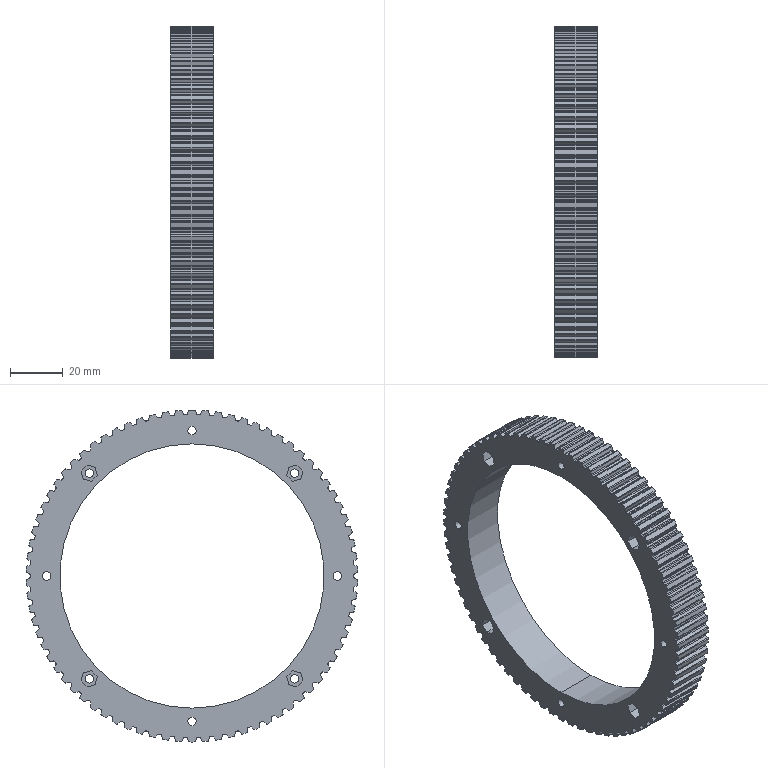Part | SolidWorks | features ICE 3, Cut 2, Chamfer 1, CirPattern 1, RefAxis 1, Revolution 1 | 1 solid | 757 faces | box 16 x 125.578 x 125.622 mm | volume 66600 mm3 | cylinder 543 | plane 214 | commonest cylinder face diameters 0.76 x184 0.82 x184 125.622 x79 122.322 x78 3.2 x16 100 x2